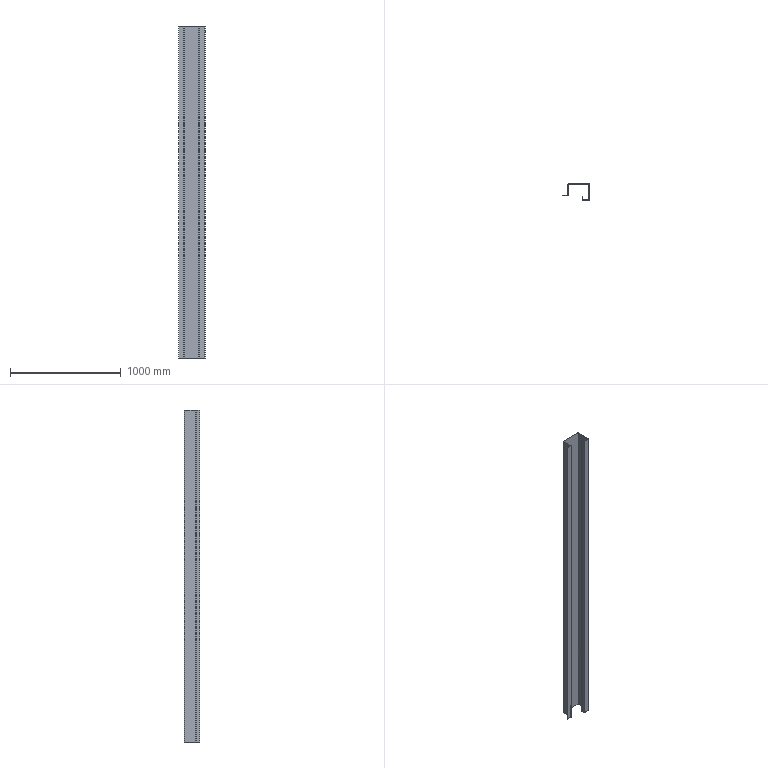Part | STEP file | SX-S31 | 1 solid | 54 faces | box 240 x 140 x 2995 mm | volume 5007531 mm3 | plane 36 | cylinder 18 | commonest cylinder face diameters 5.4 x8 0.4 x5 6.4 x5